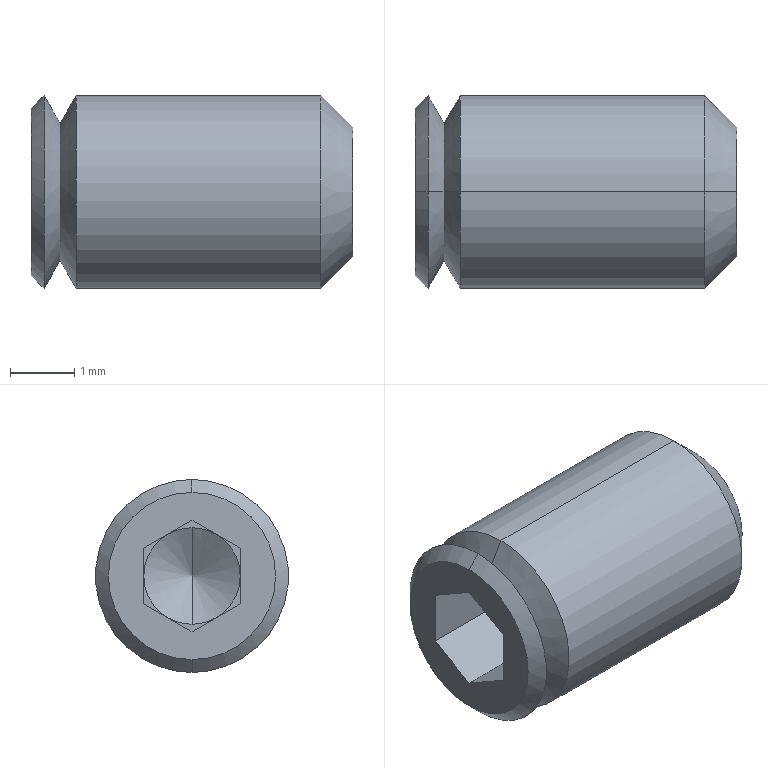Part | STEP file | GB/T 77 M3×5_M3×5 | 1 solid | 26 faces | box 5 x 3 x 3 mm | volume 30.605 mm3 | plane 14 | cone 10 | cylinder 2 | commonest cylinder face diameters 3 x2